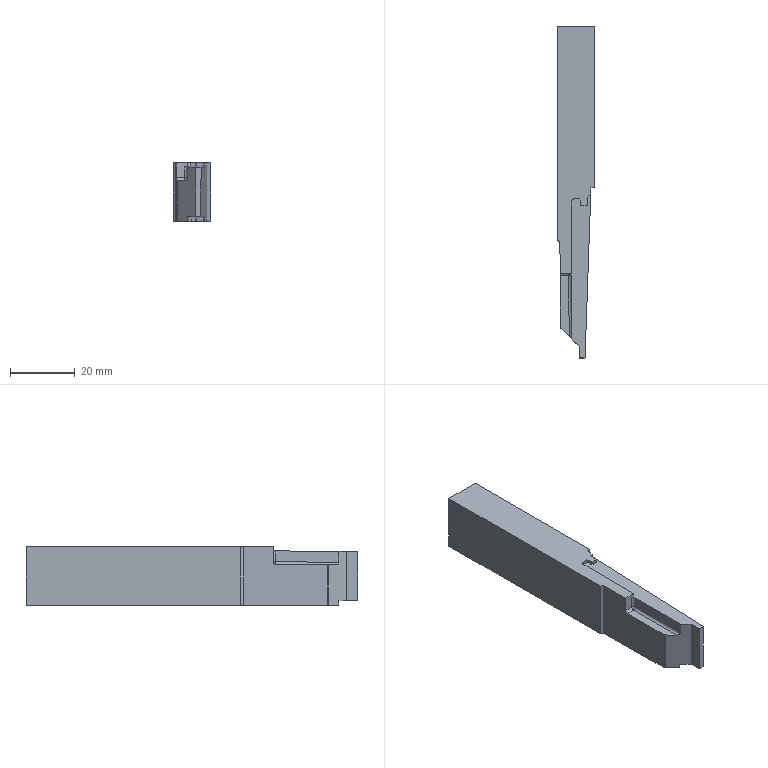Part | STEP file | 1 solid | 41 faces | box 11.534 x 102.36 x 18.001 mm | volume 17054 mm3 | plane 33 | cylinder 7 | sphere 1 | commonest cylinder face diameters 1.608 x4 2.01 x2 1.005 x1